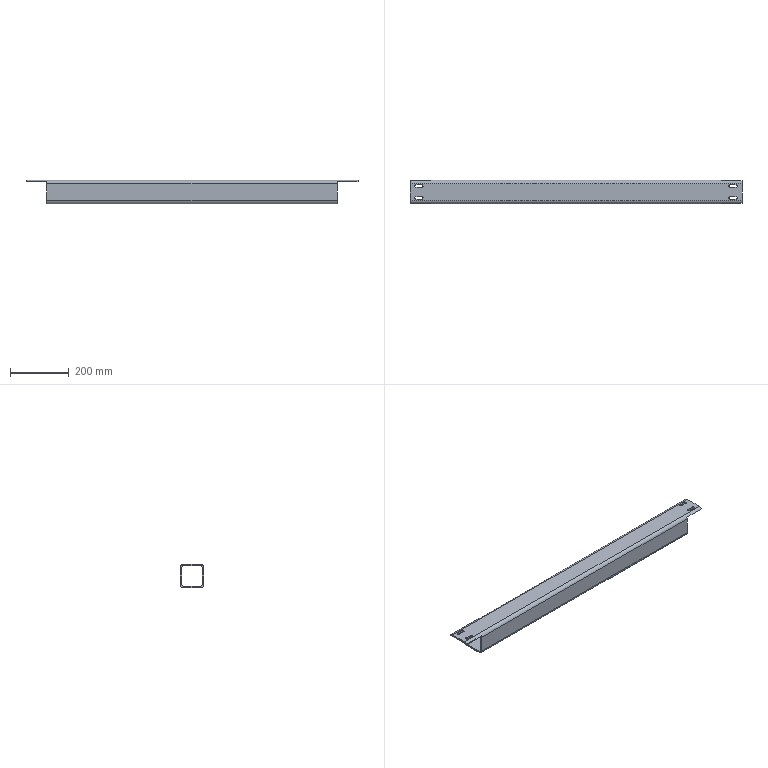Part | SolidWorks | features ICE 3, Extrusion 1 | 1 solid | 40 faces | box 1128 x 80 x 80 mm | volume 1646266 mm3 | cylinder 20 | plane 20 | commonest cylinder face diameters 8.5 x12 11.429 x4 22.857 x4
STEP:
#1=CARTESIAN_POINT('',(-439.75,-20.,34.286));
#2=VERTEX_POINT('',#1);
#3=CARTESIAN_POINT('',(-444.,-15.75,34.286));
#4=VERTEX_POINT('',#3);
#5=CARTESIAN_POINT('',(-444.,-20.,34.286));
#6=DIRECTION('',(0.,0.,1.));
#7=DIRECTION('',(1.,0.,0.));
#8=AXIS2_PLACEMENT_3D('',#5,#6,#7);
#9=CIRCLE('',#8,4.25);
#10=EDGE_CURVE('',#2,#4,#9,.T.);
#11=ORIENTED_EDGE('',*,*,#10,.F.);
#12=CARTESIAN_POINT('',(-439.75,-20.,40.));
#13=VERTEX_POINT('',#12);
#14=CARTESIAN_POINT('',(-439.75,-20.,-30.));
#15=DIRECTION('',(0.,0.,1.));
#16=VECTOR('',#15,1000.);
#17=LINE('',#14,#16);
#18=EDGE_CURVE('',#2,#13,#17,.T.);
#19=ORIENTED_EDGE('',*,*,#18,.T.);
#20=CARTESIAN_POINT('',(-444.,-15.75,40.));
#21=VERTEX_POINT('',#20);
#22=CARTESIAN_POINT('',(-444.,-20.,40.));
#23=DIRECTION('',(0.,0.,1.));
#24=DIRECTION('',(-1.,0.,0.));
#25=AXIS2_PLACEMENT_3D('',#22,#23,#24);
#26=CIRCLE('',#25,4.25);
#27=EDGE_CURVE('',#13,#21,#26,.T.);
#28=ORIENTED_EDGE('',*,*,#27,.T.);
#29=CARTESIAN_POINT('',(-444.,-15.75,-30.));
#30=DIRECTION('',(0.,0.,1.));
#31=VECTOR('',#30,1000.);
#32=LINE('',#29,#31);
#33=EDGE_CURVE('',#4,#21,#32,.T.);
#34=ORIENTED_EDGE('',*,*,#33,.F.);
#35=EDGE_LOOP('',(#11,#19,#28,#34));
#36=FACE_OUTER_BOUND('',#35,.T.);
#37=CARTESIAN_POINT('',(-444.,-20.,-30.));
#38=DIRECTION('',(0.,0.,1.));
#39=DIRECTION('',(1.,0.,0.));
#40=AXIS2_PLACEMENT_3D('',#37,#38,#39);
#41=CYLINDRICAL_SURFACE('',#40,4.25);
#42=ADVANCED_FACE('',(#36),#41,.F.);
#43=CARTESIAN_POINT('',(628.25,20.,34.286));
#44=VERTEX_POINT('',#43);
#45=CARTESIAN_POINT('',(624.,24.25,34.286));
#46=VERTEX_POINT('',#45);
#47=CARTESIAN_POINT('',(624.,20.,34.286));
#48=DIRECTION('',(0.,0.,1.));
#49=DIRECTION('',(1.,0.,0.));
#50=AXIS2_PLACEMENT_3D('',#47,#48,#49);
#51=CIRCLE('',#50,4.25);
#52=EDGE_CURVE('',#44,#46,#51,.T.);
#53=ORIENTED_EDGE('',*,*,#52,.F.);
#54=CARTESIAN_POINT('',(628.25,20.,40.));
#55=VERTEX_POINT('',#54);
#56=CARTESIAN_POINT('',(628.25,20.,-30.));
#57=DIRECTION('',(0.,0.,1.));
#58=VECTOR('',#57,1000.);
#59=LINE('',#56,#58);
#60=EDGE_CURVE('',#44,#55,#59,.T.);
#61=ORIENTED_EDGE('',*,*,#60,.T.);
#62=CARTESIAN_POINT('',(624.,24.25,40.));
#63=VERTEX_POINT('',#62);
#64=CARTESIAN_POINT('',(624.,20.,40.));
#65=DIRECTION('',(0.,0.,1.));
#66=DIRECTION('',(1.,0.,0.));
#67=AXIS2_PLACEMENT_3D('',#64,#65,#66);
#68=CIRCLE('',#67,4.25);
#69=EDGE_CURVE('',#55,#63,#68,.T.);
#70=ORIENTED_EDGE('',*,*,#69,.T.);
#71=CARTESIAN_POINT('',(624.,24.25,-30.));
#72=DIRECTION('',(0.,0.,1.));
#73=VECTOR('',#72,1000.);
#74=LINE('',#71,#73);
#75=EDGE_CURVE('',#46,#63,#74,.T.);
#76=ORIENTED_EDGE('',*,*,#75,.F.);
#77=EDGE_LOOP('',(#53,#61,#70,#76));
#78=FACE_OUTER_BOUND('',#77,.T.);
#79=CARTESIAN_POINT('',(624.,20.,-30.));
#80=DIRECTION('',(0.,0.,1.));
#81=DIRECTION('',(1.,0.,0.));
#82=AXIS2_PLACEMENT_3D('',#79,#80,#81);
#83=CYLINDRICAL_SURFACE('',#82,4.25);
#84=ADVANCED_FACE('',(#78),#83,.F.);
#85=CARTESIAN_POINT('',(628.25,-20.,34.286));
#86=VERTEX_POINT('',#85);
#87=CARTESIAN_POINT('',(624.,-15.75,34.286));
#88=VERTEX_POINT('',#87);
#89=CARTESIAN_POINT('',(624.,-20.,34.286));
#90=DIRECTION('',(0.,0.,1.));
#91=DIRECTION('',(1.,0.,0.));
#92=AXIS2_PLACEMENT_3D('',#89,#90,#91);
#93=CIRCLE('',#92,4.25);
#94=EDGE_CURVE('',#86,#88,#93,.T.);
#95=ORIENTED_EDGE('',*,*,#94,.F.);
#96=CARTESIAN_POINT('',(628.25,-20.,40.));
#97=VERTEX_POINT('',#96);
#98=CARTESIAN_POINT('',(628.25,-20.,-30.));
#99=DIRECTION('',(0.,0.,1.));
#100=VECTOR('',#99,1000.);
#101=LINE('',#98,#100);
#102=EDGE_CURVE('',#86,#97,#101,.T.);
#103=ORIENTED_EDGE('',*,*,#102,.T.);
#104=CARTESIAN_POINT('',(624.,-15.75,40.));
#105=VERTEX_POINT('',#104);
#106=CARTESIAN_POINT('',(624.,-20.,40.));
#107=DIRECTION('',(0.,0.,1.));
#108=DIRECTION('',(-1.,0.,0.));
#109=AXIS2_PLACEMENT_3D('',#106,#107,#108);
#110=CIRCLE('',#109,4.25);
#111=EDGE_CURVE('',#97,#105,#110,.T.);
#112=ORIENTED_EDGE('',*,*,#111,.T.);
#113=CARTESIAN_POINT('',(624.,-15.75,-30.));
#114=DIRECTION('',(0.,0.,1.));
#115=VECTOR('',#114,1000.);
#116=LINE('',#113,#115);
#117=EDGE_CURVE('',#88,#105,#116,.T.);
#118=ORIENTED_EDGE('',*,*,#117,.F.);
#119=EDGE_LOOP('',(#95,#103,#112,#118));
#120=FACE_OUTER_BOUND('',#119,.T.);
#121=CARTESIAN_POINT('',(624.,-20.,-30.));
#122=DIRECTION('',(0.,0.,1.));
#123=DIRECTION('',(1.,0.,0.));
#124=AXIS2_PLACEMENT_3D('',#121,#122,#123);
#125=CYLINDRICAL_SURFACE('',#124,4.25);
#126=ADVANCED_FACE('',(#120),#125,.F.);
#127=CARTESIAN_POINT('',(-439.75,20.,34.286));
#128=VERTEX_POINT('',#127);
#129=CARTESIAN_POINT('',(-444.,24.25,34.286));
#130=VERTEX_POINT('',#129);
#131=CARTESIAN_POINT('',(-444.,20.,34.286));
#132=DIRECTION('',(0.,0.,1.));
#133=DIRECTION('',(1.,0.,0.));
#134=AXIS2_PLACEMENT_3D('',#131,#132,#133);
#135=CIRCLE('',#134,4.25);
#136=EDGE_CURVE('',#128,#130,#135,.T.);
#137=ORIENTED_EDGE('',*,*,#136,.F.);
#138=CARTESIAN_POINT('',(-439.75,20.,40.));
#139=VERTEX_POINT('',#138);
#140=CARTESIAN_POINT('',(-439.75,20.,-30.));
#141=DIRECTION('',(0.,0.,1.));
#142=VECTOR('',#141,1000.);
#143=LINE('',#140,#142);
#144=EDGE_CURVE('',#128,#139,#143,.T.);
#145=ORIENTED_EDGE('',*,*,#144,.T.);
#146=CARTESIAN_POINT('',(-444.,24.25,40.));
#147=VERTEX_POINT('',#146);
#148=CARTESIAN_POINT('',(-444.,20.,40.));
#149=DIRECTION('',(0.,0.,1.));
#150=DIRECTION('',(1.,0.,0.));
#151=AXIS2_PLACEMENT_3D('',#148,#149,#150);
#152=CIRCLE('',#151,4.25);
#153=EDGE_CURVE('',#139,#147,#152,.T.);
#154=ORIENTED_EDGE('',*,*,#153,.T.);
#155=CARTESIAN_POINT('',(-444.,24.25,-30.));
#156=DIRECTION('',(0.,0.,1.));
#157=VECTOR('',#156,1000.);
#158=LINE('',#155,#157);
#159=EDGE_CURVE('',#130,#147,#158,.T.);
#160=ORIENTED_EDGE('',*,*,#159,.F.);
#161=EDGE_LOOP('',(#137,#145,#154,#160));
#162=FACE_OUTER_BOUND('',#161,.T.);
#163=CARTESIAN_POINT('',(-444.,20.,-30.));
#164=DIRECTION('',(0.,0.,1.));
#165=DIRECTION('',(1.,0.,0.));
#166=AXIS2_PLACEMENT_3D('',#163,#164,#165);
#167=CYLINDRICAL_SURFACE('',#166,4.25);
#168=ADVANCED_FACE('',(#162),#167,.F.);
#169=CARTESIAN_POINT('',(-414.,38.469,34.286));
#170=VERTEX_POINT('',#169);
#171=CARTESIAN_POINT('',(-414.,28.571,34.286));
#172=VERTEX_POINT('',#171);
#173=CARTESIAN_POINT('',(-414.,-28.571,34.286));
#174=DIRECTION('',(0.,-1.,0.));
#175=VECTOR('',#174,1000.);
#176=LINE('',#173,#175);
#177=EDGE_CURVE('',#170,#172,#176,.T.);
#178=ORIENTED_EDGE('',*,*,#177,.F.);
#179=CARTESIAN_POINT('',(-414.,40.,28.571));
#180=VERTEX_POINT('',#179);
#181=CARTESIAN_POINT('',(-414.,28.571,28.571));
#182=DIRECTION('',(1.,0.,0.));
#183=DIRECTION('',(0.,0.,-1.));
#184=AXIS2_PLACEMENT_3D('',#181,#182,#183);
#185=CIRCLE('',#184,11.429);
#186=EDGE_CURVE('',#180,#170,#185,.T.);
#187=ORIENTED_EDGE('',*,*,#186,.F.);
#188=CARTESIAN_POINT('',(-414.,40.,-28.571));
#189=VERTEX_POINT('',#188);
#190=CARTESIAN_POINT('',(-414.,40.,-28.571));
#191=DIRECTION('',(0.,0.,1.));
#192=VECTOR('',#191,1000.);
#193=LINE('',#190,#192);
#194=EDGE_CURVE('',#189,#180,#193,.T.);
#195=ORIENTED_EDGE('',*,*,#194,.F.);
#196=CARTESIAN_POINT('',(-414.,28.571,-40.));
#197=VERTEX_POINT('',#196);
#198=CARTESIAN_POINT('',(-414.,28.571,-28.571));
#199=DIRECTION('',(1.,0.,0.));
#200=DIRECTION('',(0.,0.,-1.));
#201=AXIS2_PLACEMENT_3D('',#198,#199,#200);
#202=CIRCLE('',#201,11.429);
#203=EDGE_CURVE('',#197,#189,#202,.T.);
#204=ORIENTED_EDGE('',*,*,#203,.F.);
#205=CARTESIAN_POINT('',(-414.,-28.571,-40.));
#206=VERTEX_POINT('',#205);
#207=CARTESIAN_POINT('',(-414.,-28.571,-40.));
#208=DIRECTION('',(0.,1.,0.));
#209=VECTOR('',#208,1000.);
#210=LINE('',#207,#209);
#211=EDGE_CURVE('',#206,#197,#210,.T.);
#212=ORIENTED_EDGE('',*,*,#211,.F.);
#213=CARTESIAN_POINT('',(-414.,-40.,-28.571));
#214=VERTEX_POINT('',#213);
#215=CARTESIAN_POINT('',(-414.,-28.571,-28.571));
#216=DIRECTION('',(1.,0.,0.));
#217=DIRECTION('',(0.,0.,-1.));
#218=AXIS2_PLACEMENT_3D('',#215,#216,#217);
#219=CIRCLE('',#218,11.429);
#220=EDGE_CURVE('',#214,#206,#219,.T.);
#221=ORIENTED_EDGE('',*,*,#220,.F.);
#222=CARTESIAN_POINT('',(-414.,-40.,28.571));
#223=VERTEX_POINT('',#222);
#224=CARTESIAN_POINT('',(-414.,-40.,28.571));
#225=DIRECTION('',(0.,0.,-1.));
#226=VECTOR('',#225,1000.);
#227=LINE('',#224,#226);
#228=EDGE_CURVE('',#223,#214,#227,.T.);
#229=ORIENTED_EDGE('',*,*,#228,.F.);
#230=CARTESIAN_POINT('',(-414.,-38.469,34.286));
#231=VERTEX_POINT('',#230);
#232=CARTESIAN_POINT('',(-414.,-28.571,28.571));
#233=DIRECTION('',(1.,0.,0.));
#234=DIRECTION('',(0.,0.,-1.));
#235=AXIS2_PLACEMENT_3D('',#232,#233,#234);
#236=CIRCLE('',#235,11.429);
#237=EDGE_CURVE('',#231,#223,#236,.T.);
#238=ORIENTED_EDGE('',*,*,#237,.F.);
#239=CARTESIAN_POINT('',(-414.,-28.571,34.286));
#240=VERTEX_POINT('',#239);
#241=CARTESIAN_POINT('',(-414.,-28.571,34.286));
#242=DIRECTION('',(0.,-1.,0.));
#243=VECTOR('',#242,1000.);
#244=LINE('',#241,#243);
#245=EDGE_CURVE('',#240,#231,#244,.T.);
#246=ORIENTED_EDGE('',*,*,#245,.F.);
#247=CARTESIAN_POINT('',(-414.,-34.286,28.571));
#248=VERTEX_POINT('',#247);
#249=CARTESIAN_POINT('',(-414.,-28.571,28.571));
#250=DIRECTION('',(1.,0.,0.));
#251=DIRECTION('',(0.,0.,1.));
#252=AXIS2_PLACEMENT_3D('',#249,#250,#251);
#253=CIRCLE('',#252,5.714);
#254=EDGE_CURVE('',#240,#248,#253,.T.);
#255=ORIENTED_EDGE('',*,*,#254,.T.);
#256=CARTESIAN_POINT('',(-414.,-34.286,-28.571));
#257=VERTEX_POINT('',#256);
#258=CARTESIAN_POINT('',(-414.,-34.286,-28.571));
#259=DIRECTION('',(0.,0.,-1.));
#260=VECTOR('',#259,1000.);
#261=LINE('',#258,#260);
#262=EDGE_CURVE('',#248,#257,#261,.T.);
#263=ORIENTED_EDGE('',*,*,#262,.T.);
#264=CARTESIAN_POINT('',(-414.,-28.571,-34.286));
#265=VERTEX_POINT('',#264);
#266=CARTESIAN_POINT('',(-414.,-28.571,-28.571));
#267=DIRECTION('',(1.,0.,0.));
#268=DIRECTION('',(0.,0.,1.));
#269=AXIS2_PLACEMENT_3D('',#266,#267,#268);
#270=CIRCLE('',#269,5.714);
#271=EDGE_CURVE('',#257,#265,#270,.T.);
#272=ORIENTED_EDGE('',*,*,#271,.T.);
#273=CARTESIAN_POINT('',(-414.,28.571,-34.286));
#274=VERTEX_POINT('',#273);
#275=CARTESIAN_POINT('',(-414.,28.571,-34.286));
#276=DIRECTION('',(0.,1.,0.));
#277=VECTOR('',#276,1000.);
#278=LINE('',#275,#277);
#279=EDGE_CURVE('',#265,#274,#278,.T.);
#280=ORIENTED_EDGE('',*,*,#279,.T.);
#281=CARTESIAN_POINT('',(-414.,34.286,-28.571));
#282=VERTEX_POINT('',#281);
#283=CARTESIAN_POINT('',(-414.,28.571,-28.571));
#284=DIRECTION('',(1.,0.,0.));
#285=DIRECTION('',(0.,0.,1.));
#286=AXIS2_PLACEMENT_3D('',#283,#284,#285);
#287=CIRCLE('',#286,5.714);
#288=EDGE_CURVE('',#274,#282,#287,.T.);
#289=ORIENTED_EDGE('',*,*,#288,.T.);
#290=CARTESIAN_POINT('',(-414.,34.286,28.571));
#291=VERTEX_POINT('',#290);
#292=CARTESIAN_POINT('',(-414.,34.286,28.571));
#293=DIRECTION('',(0.,0.,1.));
#294=VECTOR('',#293,1000.);
#295=LINE('',#292,#294);
#296=EDGE_CURVE('',#282,#291,#295,.T.);
#297=ORIENTED_EDGE('',*,*,#296,.T.);
#298=CARTESIAN_POINT('',(-414.,28.571,28.571));
#299=DIRECTION('',(1.,0.,0.));
#300=DIRECTION('',(0.,0.,1.));
#301=AXIS2_PLACEMENT_3D('',#298,#299,#300);
#302=CIRCLE('',#301,5.714);
#303=EDGE_CURVE('',#291,#172,#302,.T.);
#304=ORIENTED_EDGE('',*,*,#303,.T.);
#305=EDGE_LOOP('',(#178,#187,#195,#204,#212,#221,#229,#238,#246,#255,#263,#272,#280,#289,#297,#304));
#306=FACE_OUTER_BOUND('',#305,.T.);
#307=CARTESIAN_POINT('',(-414.,-28.571,-28.571));
#308=DIRECTION('',(1.,0.,0.));
#309=DIRECTION('',(0.,0.,-1.));
#310=AXIS2_PLACEMENT_3D('',#307,#308,#309);
#311=PLANE('',#310);
#312=ADVANCED_FACE('',(#306),#311,.F.);
#313=CARTESIAN_POINT('',(574.,-40.,-28.571));
#314=VERTEX_POINT('',#313);
#315=CARTESIAN_POINT('',(574.,-28.571,-40.));
#316=VERTEX_POINT('',#315);
#317=CARTESIAN_POINT('',(574.,-28.571,-28.571));
#318=DIRECTION('',(1.,0.,0.));
#319=DIRECTION('',(0.,0.,-1.));
#320=AXIS2_PLACEMENT_3D('',#317,#318,#319);
#321=CIRCLE('',#320,11.429);
#322=EDGE_CURVE('',#314,#316,#321,.T.);
#323=ORIENTED_EDGE('',*,*,#322,.F.);
#324=CARTESIAN_POINT('',(-414.,-40.,-28.571));
#325=DIRECTION('',(1.,0.,0.));
#326=VECTOR('',#325,1000.);
#327=LINE('',#324,#326);
#328=EDGE_CURVE('',#214,#314,#327,.T.);
#329=ORIENTED_EDGE('',*,*,#328,.F.);
#330=ORIENTED_EDGE('',*,*,#220,.T.);
#331=CARTESIAN_POINT('',(-414.,-28.571,-40.));
#332=DIRECTION('',(1.,0.,0.));
#333=VECTOR('',#332,1000.);
#334=LINE('',#331,#333);
#335=EDGE_CURVE('',#206,#316,#334,.T.);
#336=ORIENTED_EDGE('',*,*,#335,.T.);
#337=EDGE_LOOP('',(#323,#329,#330,#336));
#338=FACE_OUTER_BOUND('',#337,.T.);
#339=CARTESIAN_POINT('',(-414.,-28.571,-28.571));
#340=DIRECTION('',(1.,0.,0.));
#341=DIRECTION('',(0.,0.,-1.));
#342=AXIS2_PLACEMENT_3D('',#339,#340,#341);
#343=CYLINDRICAL_SURFACE('',#342,11.429);
#344=ADVANCED_FACE('',(#338),#343,.T.);
#345=CARTESIAN_POINT('',(574.,-40.,28.571));
#346=VERTEX_POINT('',#345);
#347=CARTESIAN_POINT('',(574.,-40.,28.571));
#348=DIRECTION('',(0.,0.,-1.));
#349=VECTOR('',#348,1000.);
#350=LINE('',#347,#349);
#351=EDGE_CURVE('',#346,#314,#350,.T.);
#352=ORIENTED_EDGE('',*,*,#351,.F.);
#353=CARTESIAN_POINT('',(-414.,-40.,28.571));
#354=DIRECTION('',(1.,0.,0.));
#355=VECTOR('',#354,1000.);
#356=LINE('',#353,#355);
#357=EDGE_CURVE('',#223,#346,#356,.T.);
#358=ORIENTED_EDGE('',*,*,#357,.F.);
#359=ORIENTED_EDGE('',*,*,#228,.T.);
#360=ORIENTED_EDGE('',*,*,#328,.T.);
#361=EDGE_LOOP('',(#352,#358,#359,#360));
#362=FACE_OUTER_BOUND('',#361,.T.);
#363=CARTESIAN_POINT('',(-414.,-40.,28.571));
#364=DIRECTION('',(0.,-1.,0.));
#365=DIRECTION('',(0.,0.,-1.));
#366=AXIS2_PLACEMENT_3D('',#363,#364,#365);
#367=PLANE('',#366);
#368=ADVANCED_FACE('',(#362),#367,.T.);
#369=CARTESIAN_POINT('',(574.,-38.469,34.286));
#370=VERTEX_POINT('',#369);
#371=CARTESIAN_POINT('',(574.,-28.571,28.571));
#372=DIRECTION('',(1.,0.,0.));
#373=DIRECTION('',(0.,0.,-1.));
#374=AXIS2_PLACEMENT_3D('',#371,#372,#373);
#375=CIRCLE('',#374,11.429);
#376=EDGE_CURVE('',#370,#346,#375,.T.);
#377=ORIENTED_EDGE('',*,*,#376,.F.);
#378=CARTESIAN_POINT('',(644.,-38.469,34.286));
#379=VERTEX_POINT('',#378);
#380=CARTESIAN_POINT('',(644.,-38.469,34.286));
#381=DIRECTION('',(-1.,0.,0.));
#382=VECTOR('',#381,1000.);
#383=LINE('',#380,#382);
#384=EDGE_CURVE('',#379,#370,#383,.T.);
#385=ORIENTED_EDGE('',*,*,#384,.F.);
#386=CARTESIAN_POINT('',(644.,-28.571,40.));
#387=VERTEX_POINT('',#386);
#388=CARTESIAN_POINT('',(644.,-28.571,28.571));
#389=DIRECTION('',(1.,0.,0.));
#390=DIRECTION('',(0.,0.,-1.));
#391=AXIS2_PLACEMENT_3D('',#388,#389,#390);
#392=CIRCLE('',#391,11.429);
#393=EDGE_CURVE('',#387,#379,#392,.T.);
#394=ORIENTED_EDGE('',*,*,#393,.F.);
#395=CARTESIAN_POINT('',(-484.,-28.571,40.));
#396=VERTEX_POINT('',#395);
#397=CARTESIAN_POINT('',(-414.,-28.571,40.));
#398=DIRECTION('',(1.,0.,0.));
#399=VECTOR('',#398,1000.);
#400=LINE('',#397,#399);
#401=EDGE_CURVE('',#396,#387,#400,.T.);
#402=ORIENTED_EDGE('',*,*,#401,.F.);
#403=CARTESIAN_POINT('',(-484.,-38.469,34.286));
#404=VERTEX_POINT('',#403);
#405=CARTESIAN_POINT('',(-484.,-28.571,28.571));
#406=DIRECTION('',(-1.,0.,0.));
#407=DIRECTION('',(0.,0.,1.));
#408=AXIS2_PLACEMENT_3D('',#405,#406,#407);
#409=CIRCLE('',#408,11.429);
#410=EDGE_CURVE('',#404,#396,#409,.T.);
#411=ORIENTED_EDGE('',*,*,#410,.F.);
#412=CARTESIAN_POINT('',(-484.,-38.469,34.286));
#413=DIRECTION('',(1.,0.,0.));
#414=VECTOR('',#413,1000.);
#415=LINE('',#412,#414);
#416=EDGE_CURVE('',#404,#231,#415,.T.);
#417=ORIENTED_EDGE('',*,*,#416,.T.);
#418=ORIENTED_EDGE('',*,*,#237,.T.);
#419=ORIENTED_EDGE('',*,*,#357,.T.);
#420=EDGE_LOOP('',(#377,#385,#394,#402,#411,#417,#418,#419));
#421=FACE_OUTER_BOUND('',#420,.T.);
#422=CARTESIAN_POINT('',(-414.,-28.571,28.571));
#423=DIRECTION('',(1.,0.,0.));
#424=DIRECTION('',(0.,0.,-1.));
#425=AXIS2_PLACEMENT_3D('',#422,#423,#424);
#426=CYLINDRICAL_SURFACE('',#425,11.429);
#427=ADVANCED_FACE('',(#421),#426,.T.);
#428=CARTESIAN_POINT('',(-464.,-15.75,40.));
#429=VERTEX_POINT('',#428);
#430=CARTESIAN_POINT('',(-464.,-24.25,40.));
#431=VERTEX_POINT('',#430);
#432=CARTESIAN_POINT('',(-464.,-20.,40.));
#433=DIRECTION('',(0.,0.,1.));
#434=DIRECTION('',(-1.,0.,0.));
#435=AXIS2_PLACEMENT_3D('',#432,#433,#434);
#436=CIRCLE('',#435,4.25);
#437=EDGE_CURVE('',#429,#431,#436,.T.);
#438=ORIENTED_EDGE('',*,*,#437,.F.);
#439=CARTESIAN_POINT('',(-464.,-15.75,40.));
#440=DIRECTION('',(-1.,0.,0.));
#441=VECTOR('',#440,1000.);
#442=LINE('',#439,#441);
#443=EDGE_CURVE('',#21,#429,#442,.T.);
#444=ORIENTED_EDGE('',*,*,#443,.F.);
#445=ORIENTED_EDGE('',*,*,#27,.F.);
#446=CARTESIAN_POINT('',(-444.,-24.25,40.));
#447=VERTEX_POINT('',#446);
#448=CARTESIAN_POINT('',(-444.,-20.,40.));
#449=DIRECTION('',(0.,0.,1.));
#450=DIRECTION('',(-1.,0.,0.));
#451=AXIS2_PLACEMENT_3D('',#448,#449,#450);
#452=CIRCLE('',#451,4.25);
#453=EDGE_CURVE('',#447,#13,#452,.T.);
#454=ORIENTED_EDGE('',*,*,#453,.F.);
#455=CARTESIAN_POINT('',(-464.,-24.25,40.));
#456=DIRECTION('',(1.,0.,0.));
#457=VECTOR('',#456,1000.);
#458=LINE('',#455,#457);
#459=EDGE_CURVE('',#431,#447,#458,.T.);
#460=ORIENTED_EDGE('',*,*,#459,.F.);
#461=EDGE_LOOP('',(#438,#444,#445,#454,#460));
#462=FACE_BOUND('',#461,.T.);
#463=CARTESIAN_POINT('',(604.,24.25,40.));
#464=VERTEX_POINT('',#463);
#465=CARTESIAN_POINT('',(604.,15.75,40.));
#466=VERTEX_POINT('',#465);
#467=CARTESIAN_POINT('',(604.,20.,40.));
#468=DIRECTION('',(0.,0.,1.));
#469=DIRECTION('',(1.,0.,0.));
#470=AXIS2_PLACEMENT_3D('',#467,#468,#469);
#471=CIRCLE('',#470,4.25);
#472=EDGE_CURVE('',#464,#466,#471,.T.);
#473=ORIENTED_EDGE('',*,*,#472,.F.);
#474=CARTESIAN_POINT('',(604.,24.25,40.));
#475=DIRECTION('',(-1.,0.,0.));
#476=VECTOR('',#475,1000.);
#477=LINE('',#474,#476);
#478=EDGE_CURVE('',#63,#464,#477,.T.);
#479=ORIENTED_EDGE('',*,*,#478,.F.);
#480=ORIENTED_EDGE('',*,*,#69,.F.);
#481=CARTESIAN_POINT('',(624.,15.75,40.));
#482=VERTEX_POINT('',#481);
#483=CARTESIAN_POINT('',(624.,20.,40.));
#484=DIRECTION('',(0.,0.,1.));
#485=DIRECTION('',(1.,0.,0.));
#486=AXIS2_PLACEMENT_3D('',#483,#484,#485);
#487=CIRCLE('',#486,4.25);
#488=EDGE_CURVE('',#482,#55,#487,.T.);
#489=ORIENTED_EDGE('',*,*,#488,.F.);
#490=CARTESIAN_POINT('',(604.,15.75,40.));
#491=DIRECTION('',(1.,0.,0.));
#492=VECTOR('',#491,1000.);
#493=LINE('',#490,#492);
#494=EDGE_CURVE('',#466,#482,#493,.T.);
#495=ORIENTED_EDGE('',*,*,#494,.F.);
#496=EDGE_LOOP('',(#473,#479,#480,#489,#495));
#497=FACE_BOUND('',#496,.T.);
#498=CARTESIAN_POINT('',(604.,-15.75,40.));
#499=VERTEX_POINT('',#498);
#500=CARTESIAN_POINT('',(604.,-24.25,40.));
#501=VERTEX_POINT('',#500);
#502=CARTESIAN_POINT('',(604.,-20.,40.));
#503=DIRECTION('',(0.,0.,1.));
#504=DIRECTION('',(-1.,0.,0.));
#505=AXIS2_PLACEMENT_3D('',#502,#503,#504);
#506=CIRCLE('',#505,4.25);
#507=EDGE_CURVE('',#499,#501,#506,.T.);
#508=ORIENTED_EDGE('',*,*,#507,.F.);
#509=CARTESIAN_POINT('',(604.,-15.75,40.));
#510=DIRECTION('',(-1.,0.,0.));
#511=VECTOR('',#510,1000.);
#512=LINE('',#509,#511);
#513=EDGE_CURVE('',#105,#499,#512,.T.);
#514=ORIENTED_EDGE('',*,*,#513,.F.);
#515=ORIENTED_EDGE('',*,*,#111,.F.);
#516=CARTESIAN_POINT('',(624.,-24.25,40.));
#517=VERTEX_POINT('',#516);
#518=CARTESIAN_POINT('',(624.,-20.,40.));
#519=DIRECTION('',(0.,0.,1.));
#520=DIRECTION('',(-1.,0.,0.));
#521=AXIS2_PLACEMENT_3D('',#518,#519,#520);
#522=CIRCLE('',#521,4.25);
#523=EDGE_CURVE('',#517,#97,#522,.T.);
#524=ORIENTED_EDGE('',*,*,#523,.F.);
#525=CARTESIAN_POINT('',(604.,-24.25,40.));
#526=DIRECTION('',(1.,0.,0.));
#527=VECTOR('',#526,1000.);
#528=LINE('',#525,#527);
#529=EDGE_CURVE('',#501,#517,#528,.T.);
#530=ORIENTED_EDGE('',*,*,#529,.F.);
#531=EDGE_LOOP('',(#508,#514,#515,#524,#530));
#532=FACE_BOUND('',#531,.T.);
#533=CARTESIAN_POINT('',(-464.,24.25,40.));
#534=VERTEX_POINT('',#533);
#535=CARTESIAN_POINT('',(-464.,15.75,40.));
#536=VERTEX_POINT('',#535);
#537=CARTESIAN_POINT('',(-464.,20.,40.));
#538=DIRECTION('',(0.,0.,1.));
#539=DIRECTION('',(1.,0.,0.));
#540=AXIS2_PLACEMENT_3D('',#537,#538,#539);
#541=CIRCLE('',#540,4.25);
#542=EDGE_CURVE('',#534,#536,#541,.T.);
#543=ORIENTED_EDGE('',*,*,#542,.F.);
#544=CARTESIAN_POINT('',(-464.,24.25,40.));
#545=DIRECTION('',(-1.,0.,0.));
#546=VECTOR('',#545,1000.);
#547=LINE('',#544,#546);
#548=EDGE_CURVE('',#147,#534,#547,.T.);
#549=ORIENTED_EDGE('',*,*,#548,.F.);
#550=ORIENTED_EDGE('',*,*,#153,.F.);
#551=CARTESIAN_POINT('',(-444.,15.75,40.));
#552=VERTEX_POINT('',#551);
#553=CARTESIAN_POINT('',(-444.,20.,40.));
#554=DIRECTION('',(0.,0.,1.));
#555=DIRECTION('',(1.,0.,0.));
#556=AXIS2_PLACEMENT_3D('',#553,#554,#555);
#557=CIRCLE('',#556,4.25);
#558=EDGE_CURVE('',#552,#139,#557,.T.);
#559=ORIENTED_EDGE('',*,*,#558,.F.);
#560=CARTESIAN_POINT('',(-464.,15.75,40.));
#561=DIRECTION('',(1.,0.,0.));
#562=VECTOR('',#561,1000.);
#563=LINE('',#560,#562);
#564=EDGE_CURVE('',#536,#552,#563,.T.);
#565=ORIENTED_EDGE('',*,*,#564,.F.);
#566=EDGE_LOOP('',(#543,#549,#550,#559,#565));
#567=FACE_BOUND('',#566,.T.);
#568=ORIENTED_EDGE('',*,*,#401,.T.);
#569=CARTESIAN_POINT('',(644.,28.571,40.));
#570=VERTEX_POINT('',#569);
#571=CARTESIAN_POINT('',(644.,28.571,40.));
#572=DIRECTION('',(0.,-1.,0.));
#573=VECTOR('',#572,1000.);
#574=LINE('',#571,#573);
#575=EDGE_CURVE('',#570,#387,#574,.T.);
#576=ORIENTED_EDGE('',*,*,#575,.F.);
#577=CARTESIAN_POINT('',(-484.,28.571,40.));
#578=VERTEX_POINT('',#577);
#579=CARTESIAN_POINT('',(-414.,28.571,40.));
#580=DIRECTION('',(1.,0.,0.));
#581=VECTOR('',#580,1000.);
#582=LINE('',#579,#581);
#583=EDGE_CURVE('',#578,#570,#582,.T.);
#584=ORIENTED_EDGE('',*,*,#583,.F.);
#585=CARTESIAN_POINT('',(-484.,-28.571,40.));
#586=DIRECTION('',(0.,1.,0.));
#587=VECTOR('',#586,1000.);
#588=LINE('',#585,#587);
#589=EDGE_CURVE('',#396,#578,#588,.T.);
#590=ORIENTED_EDGE('',*,*,#589,.F.);
#591=EDGE_LOOP('',(#568,#576,#584,#590));
#592=FACE_OUTER_BOUND('',#591,.T.);
#593=CARTESIAN_POINT('',(-414.,28.571,40.));
#594=DIRECTION('',(0.,0.,1.));
#595=DIRECTION('',(1.,0.,0.));
#596=AXIS2_PLACEMENT_3D('',#593,#594,#595);
#597=PLANE('',#596);
#598=ADVANCED_FACE('',(#462,#497,#532,#567,#592),#597,.T.);
#599=CARTESIAN_POINT('',(574.,40.,28.571));
#600=VERTEX_POINT('',#599);
#601=CARTESIAN_POINT('',(574.,38.469,34.286));
#602=VERTEX_POINT('',#601);
#603=CARTESIAN_POINT('',(574.,28.571,28.571));
#604=DIRECTION('',(1.,0.,0.));
#605=DIRECTION('',(0.,0.,-1.));
#606=AXIS2_PLACEMENT_3D('',#603,#604,#605);
#607=CIRCLE('',#606,11.429);
#608=EDGE_CURVE('',#600,#602,#607,.T.);
#609=ORIENTED_EDGE('',*,*,#608,.F.);
#610=CARTESIAN_POINT('',(-414.,40.,28.571));
#611=DIRECTION('',(1.,0.,0.));
#612=VECTOR('',#611,1000.);
#613=LINE('',#610,#612);
#614=EDGE_CURVE('',#180,#600,#613,.T.);
#615=ORIENTED_EDGE('',*,*,#614,.F.);
#616=ORIENTED_EDGE('',*,*,#186,.T.);
#617=CARTESIAN_POINT('',(-484.,38.469,34.286));
#618=VERTEX_POINT('',#617);
#619=CARTESIAN_POINT('',(-484.,38.469,34.286));
#620=DIRECTION('',(1.,0.,0.));
#621=VECTOR('',#620,1000.);
#622=LINE('',#619,#621);
#623=EDGE_CURVE('',#618,#170,#622,.T.);
#624=ORIENTED_EDGE('',*,*,#623,.F.);
#625=CARTESIAN_POINT('',(-484.,28.571,28.571));
#626=DIRECTION('',(-1.,0.,0.));
#627=DIRECTION('',(0.,0.,1.));
#628=AXIS2_PLACEMENT_3D('',#625,#626,#627);
#629=CIRCLE('',#628,11.429);
#630=EDGE_CURVE('',#578,#618,#629,.T.);
#631=ORIENTED_EDGE('',*,*,#630,.F.);
#632=ORIENTED_EDGE('',*,*,#583,.T.);
#633=CARTESIAN_POINT('',(644.,38.469,34.286));
#634=VERTEX_POINT('',#633);
#635=CARTESIAN_POINT('',(644.,28.571,28.571));
#636=DIRECTION('',(1.,0.,0.));
#637=DIRECTION('',(0.,0.,-1.));
#638=AXIS2_PLACEMENT_3D('',#635,#636,#637);
#639=CIRCLE('',#638,11.429);
#640=EDGE_CURVE('',#634,#570,#639,.T.);
#641=ORIENTED_EDGE('',*,*,#640,.F.);
#642=CARTESIAN_POINT('',(644.,38.469,34.286));
#643=DIRECTION('',(-1.,0.,0.));
#644=VECTOR('',#643,1000.);
#645=LINE('',#642,#644);
#646=EDGE_CURVE('',#634,#602,#645,.T.);
#647=ORIENTED_EDGE('',*,*,#646,.T.);
#648=EDGE_LOOP('',(#609,#615,#616,#624,#631,#632,#641,#647));
#649=FACE_OUTER_BOUND('',#648,.T.);
#650=CARTESIAN_POINT('',(-414.,28.571,28.571));
#651=DIRECTION('',(1.,0.,0.));
#652=DIRECTION('',(0.,0.,-1.));
#653=AXIS2_PLACEMENT_3D('',#650,#651,#652);
#654=CYLINDRICAL_SURFACE('',#653,11.429);
#655=ADVANCED_FACE('',(#649),#654,.T.);
#656=CARTESIAN_POINT('',(574.,40.,-28.571));
#657=VERTEX_POINT('',#656);
#658=CARTESIAN_POINT('',(574.,40.,-28.571));
#659=DIRECTION('',(0.,0.,1.));
#660=VECTOR('',#659,1000.);
#661=LINE('',#658,#660);
#662=EDGE_CURVE('',#657,#600,#661,.T.);
#663=ORIENTED_EDGE('',*,*,#662,.F.);
#664=CARTESIAN_POINT('',(-414.,40.,-28.571));
#665=DIRECTION('',(1.,0.,0.));
#666=VECTOR('',#665,1000.);
#667=LINE('',#664,#666);
#668=EDGE_CURVE('',#189,#657,#667,.T.);
#669=ORIENTED_EDGE('',*,*,#668,.F.);
#670=ORIENTED_EDGE('',*,*,#194,.T.);
#671=ORIENTED_EDGE('',*,*,#614,.T.);
#672=EDGE_LOOP('',(#663,#669,#670,#671));
#673=FACE_OUTER_BOUND('',#672,.T.);
#674=CARTESIAN_POINT('',(-414.,40.,-28.571));
#675=DIRECTION('',(0.,1.,0.));
#676=DIRECTION('',(0.,0.,1.));
#677=AXIS2_PLACEMENT_3D('',#674,#675,#676);
#678=PLANE('',#677);
#679=ADVANCED_FACE('',(#673),#678,.T.);
#680=CARTESIAN_POINT('',(574.,28.571,-40.));
#681=VERTEX_POINT('',#680);
#682=CARTESIAN_POINT('',(574.,28.571,-28.571));
#683=DIRECTION('',(1.,0.,0.));
#684=DIRECTION('',(0.,0.,-1.));
#685=AXIS2_PLACEMENT_3D('',#682,#683,#684);
#686=CIRCLE('',#685,11.429);
#687=EDGE_CURVE('',#681,#657,#686,.T.);
#688=ORIENTED_EDGE('',*,*,#687,.F.);
#689=CARTESIAN_POINT('',(-414.,28.571,-40.));
#690=DIRECTION('',(1.,0.,0.));
#691=VECTOR('',#690,1000.);
#692=LINE('',#689,#691);
#693=EDGE_CURVE('',#197,#681,#692,.T.);
#694=ORIENTED_EDGE('',*,*,#693,.F.);
#695=ORIENTED_EDGE('',*,*,#203,.T.);
#696=ORIENTED_EDGE('',*,*,#668,.T.);
#697=EDGE_LOOP('',(#688,#694,#695,#696));
#698=FACE_OUTER_BOUND('',#697,.T.);
#699=CARTESIAN_POINT('',(-414.,28.571,-28.571));
#700=DIRECTION('',(1.,0.,0.));
#701=DIRECTION('',(0.,0.,-1.));
#702=AXIS2_PLACEMENT_3D('',#699,#700,#701);
#703=CYLINDRICAL_SURFACE('',#702,11.429);
#704=ADVANCED_FACE('',(#698),#703,.T.);
#705=CARTESIAN_POINT('',(574.,-28.571,-40.));
#706=DIRECTION('',(0.,1.,0.));
#707=VECTOR('',#706,1000.);
#708=LINE('',#705,#707);
#709=EDGE_CURVE('',#316,#681,#708,.T.);
#710=ORIENTED_EDGE('',*,*,#709,.F.);
#711=ORIENTED_EDGE('',*,*,#335,.F.);
#712=ORIENTED_EDGE('',*,*,#211,.T.);
#713=ORIENTED_EDGE('',*,*,#693,.T.);
#714=EDGE_LOOP('',(#710,#711,#712,#713));
#715=FACE_OUTER_BOUND('',#714,.T.);
#716=CARTESIAN_POINT('',(-414.,-28.571,-40.));
#717=DIRECTION('',(0.,0.,-1.));
#718=DIRECTION('',(-1.,0.,0.));
#719=AXIS2_PLACEMENT_3D('',#716,#717,#718);
#720=PLANE('',#719);
#721=ADVANCED_FACE('',(#715),#720,.T.);
#722=CARTESIAN_POINT('',(574.,-28.571,34.286));
#723=VERTEX_POINT('',#722);
#724=CARTESIAN_POINT('',(574.,28.571,34.286));
#725=DIRECTION('',(0.,1.,0.));
#726=VECTOR('',#725,1000.);
#727=LINE('',#724,#726);
#728=EDGE_CURVE('',#370,#723,#727,.T.);
#729=ORIENTED_EDGE('',*,*,#728,.F.);
#730=ORIENTED_EDGE('',*,*,#376,.T.);
#731=ORIENTED_EDGE('',*,*,#351,.T.);
#732=ORIENTED_EDGE('',*,*,#322,.T.);
#733=ORIENTED_EDGE('',*,*,#709,.T.);
#734=ORIENTED_EDGE('',*,*,#687,.T.);
#735=ORIENTED_EDGE('',*,*,#662,.T.);
#736=ORIENTED_EDGE('',*,*,#608,.T.);
#737=CARTESIAN_POINT('',(574.,28.571,34.286));
#738=VERTEX_POINT('',#737);
#739=CARTESIAN_POINT('',(574.,28.571,34.286));
#740=DIRECTION('',(0.,1.,0.));
#741=VECTOR('',#740,1000.);
#742=LINE('',#739,#741);
#743=EDGE_CURVE('',#738,#602,#742,.T.);
#744=ORIENTED_EDGE('',*,*,#743,.F.);
#745=CARTESIAN_POINT('',(574.,34.286,28.571));
#746=VERTEX_POINT('',#745);
#747=CARTESIAN_POINT('',(574.,28.571,28.571));
#748=DIRECTION('',(1.,0.,0.));
#749=DIRECTION('',(0.,0.,1.));
#750=AXIS2_PLACEMENT_3D('',#747,#748,#749);
#751=CIRCLE('',#750,5.714);
#752=EDGE_CURVE('',#746,#738,#751,.T.);
#753=ORIENTED_EDGE('',*,*,#752,.F.);
#754=CARTESIAN_POINT('',(574.,34.286,-28.571));
#755=VERTEX_POINT('',#754);
#756=CARTESIAN_POINT('',(574.,34.286,28.571));
#757=DIRECTION('',(0.,0.,1.));
#758=VECTOR('',#757,1000.);
#759=LINE('',#756,#758);
#760=EDGE_CURVE('',#755,#746,#759,.T.);
#761=ORIENTED_EDGE('',*,*,#760,.F.);
#762=CARTESIAN_POINT('',(574.,28.571,-34.286));
#763=VERTEX_POINT('',#762);
#764=CARTESIAN_POINT('',(574.,28.571,-28.571));
#765=DIRECTION('',(1.,0.,0.));
#766=DIRECTION('',(0.,0.,1.));
#767=AXIS2_PLACEMENT_3D('',#764,#765,#766);
#768=CIRCLE('',#767,5.714);
#769=EDGE_CURVE('',#763,#755,#768,.T.);
#770=ORIENTED_EDGE('',*,*,#769,.F.);
#771=CARTESIAN_POINT('',(574.,-28.571,-34.286));
#772=VERTEX_POINT('',#771);
#773=CARTESIAN_POINT('',(574.,28.571,-34.286));
#774=DIRECTION('',(0.,1.,0.));
#775=VECTOR('',#774,1000.);
#776=LINE('',#773,#775);
#777=EDGE_CURVE('',#772,#763,#776,.T.);
#778=ORIENTED_EDGE('',*,*,#777,.F.);
#779=CARTESIAN_POINT('',(574.,-34.286,-28.571));
#780=VERTEX_POINT('',#779);
#781=CARTESIAN_POINT('',(574.,-28.571,-28.571));
#782=DIRECTION('',(1.,0.,0.));
#783=DIRECTION('',(0.,0.,1.));
#784=AXIS2_PLACEMENT_3D('',#781,#782,#783);
#785=CIRCLE('',#784,5.714);
#786=EDGE_CURVE('',#780,#772,#785,.T.);
#787=ORIENTED_EDGE('',*,*,#786,.F.);
#788=CARTESIAN_POINT('',(574.,-34.286,28.571));
#789=VERTEX_POINT('',#788);
#790=CARTESIAN_POINT('',(574.,-34.286,-28.571));
#791=DIRECTION('',(0.,0.,-1.));
#792=VECTOR('',#791,1000.);
#793=LINE('',#790,#792);
#794=EDGE_CURVE('',#789,#780,#793,.T.);
#795=ORIENTED_EDGE('',*,*,#794,.F.);
#796=CARTESIAN_POINT('',(574.,-28.571,28.571));
#797=DIRECTION('',(1.,0.,0.));
#798=DIRECTION('',(0.,0.,1.));
#799=AXIS2_PLACEMENT_3D('',#796,#797,#798);
#800=CIRCLE('',#799,5.714);
#801=EDGE_CURVE('',#723,#789,#800,.T.);
#802=ORIENTED_EDGE('',*,*,#801,.F.);
#803=EDGE_LOOP('',(#729,#730,#731,#732,#733,#734,#735,#736,#744,#753,#761,#770,#778,#787,#795,#802));
#804=FACE_OUTER_BOUND('',#803,.T.);
#805=CARTESIAN_POINT('',(574.,-28.571,-28.571));
#806=DIRECTION('',(1.,0.,0.));
#807=DIRECTION('',(0.,0.,-1.));
#808=AXIS2_PLACEMENT_3D('',#805,#806,#807);
#809=PLANE('',#808);
#810=ADVANCED_FACE('',(#804),#809,.T.);
#811=ORIENTED_EDGE('',*,*,#801,.T.);
#812=CARTESIAN_POINT('',(-414.,-34.286,28.571));
#813=DIRECTION('',(1.,0.,0.));
#814=VECTOR('',#813,1000.);
#815=LINE('',#812,#814);
#816=EDGE_CURVE('',#248,#789,#815,.T.);
#817=ORIENTED_EDGE('',*,*,#816,.F.);
#818=ORIENTED_EDGE('',*,*,#254,.F.);
#819=CARTESIAN_POINT('',(-414.,-28.571,34.286));
#820=DIRECTION('',(1.,0.,0.));
#821=VECTOR('',#820,1000.);
#822=LINE('',#819,#821);
#823=EDGE_CURVE('',#240,#723,#822,.T.);
#824=ORIENTED_EDGE('',*,*,#823,.T.);
#825=EDGE_LOOP('',(#811,#817,#818,#824));
#826=FACE_OUTER_BOUND('',#825,.T.);
#827=CARTESIAN_POINT('',(-414.,-28.571,28.571));
#828=DIRECTION('',(1.,0.,0.));
#829=DIRECTION('',(0.,0.,-1.));
#830=AXIS2_PLACEMENT_3D('',#827,#828,#829);
#831=CYLINDRICAL_SURFACE('',#830,5.714);
#832=ADVANCED_FACE('',(#826),#831,.F.);
#833=CARTESIAN_POINT('',(-464.,-15.75,34.286));
#834=VERTEX_POINT('',#833);
#835=CARTESIAN_POINT('',(-414.,-15.75,34.286));
#836=DIRECTION('',(-1.,0.,0.));
#837=VECTOR('',#836,1000.);
#838=LINE('',#835,#837);
#839=EDGE_CURVE('',#4,#834,#838,.T.);
#840=ORIENTED_EDGE('',*,*,#839,.T.);
#841=CARTESIAN_POINT('',(-464.,-24.25,34.286));
#842=VERTEX_POINT('',#841);
#843=CARTESIAN_POINT('',(-464.,-20.,34.286));
#844=DIRECTION('',(0.,0.,1.));
#845=DIRECTION('',(1.,0.,0.));
#846=AXIS2_PLACEMENT_3D('',#843,#844,#845);
#847=CIRCLE('',#846,4.25);
#848=EDGE_CURVE('',#834,#842,#847,.T.);
#849=ORIENTED_EDGE('',*,*,#848,.T.);
#850=CARTESIAN_POINT('',(-444.,-24.25,34.286));
#851=VERTEX_POINT('',#850);
#852=CARTESIAN_POINT('',(-414.,-24.25,34.286));
#853=DIRECTION('',(1.,0.,0.));
#854=VECTOR('',#853,1000.);
#855=LINE('',#852,#854);
#856=EDGE_CURVE('',#842,#851,#855,.T.);
#857=ORIENTED_EDGE('',*,*,#856,.T.);
#858=CARTESIAN_POINT('',(-444.,-20.,34.286));
#859=DIRECTION('',(0.,0.,1.));
#860=DIRECTION('',(1.,0.,0.));
#861=AXIS2_PLACEMENT_3D('',#858,#859,#860);
#862=CIRCLE('',#861,4.25);
#863=EDGE_CURVE('',#851,#2,#862,.T.);
#864=ORIENTED_EDGE('',*,*,#863,.T.);
#865=ORIENTED_EDGE('',*,*,#10,.T.);
#866=EDGE_LOOP('',(#840,#849,#857,#864,#865));
#867=FACE_BOUND('',#866,.T.);
#868=CARTESIAN_POINT('',(604.,24.25,34.286));
#869=VERTEX_POINT('',#868);
#870=CARTESIAN_POINT('',(-414.,24.25,34.286));
#871=DIRECTION('',(-1.,0.,0.));
#872=VECTOR('',#871,1000.);
#873=LINE('',#870,#872);
#874=EDGE_CURVE('',#46,#869,#873,.T.);
#875=ORIENTED_EDGE('',*,*,#874,.T.);
#876=CARTESIAN_POINT('',(604.,15.75,34.286));
#877=VERTEX_POINT('',#876);
#878=CARTESIAN_POINT('',(604.,20.,34.286));
#879=DIRECTION('',(0.,0.,1.));
#880=DIRECTION('',(1.,0.,0.));
#881=AXIS2_PLACEMENT_3D('',#878,#879,#880);
#882=CIRCLE('',#881,4.25);
#883=EDGE_CURVE('',#869,#877,#882,.T.);
#884=ORIENTED_EDGE('',*,*,#883,.T.);
#885=CARTESIAN_POINT('',(624.,15.75,34.286));
#886=VERTEX_POINT('',#885);
#887=CARTESIAN_POINT('',(-414.,15.75,34.286));
#888=DIRECTION('',(1.,0.,0.));
#889=VECTOR('',#888,1000.);
#890=LINE('',#887,#889);
#891=EDGE_CURVE('',#877,#886,#890,.T.);
#892=ORIENTED_EDGE('',*,*,#891,.T.);
#893=CARTESIAN_POINT('',(624.,20.,34.286));
#894=DIRECTION('',(0.,0.,1.));
#895=DIRECTION('',(1.,0.,0.));
#896=AXIS2_PLACEMENT_3D('',#893,#894,#895);
#897=CIRCLE('',#896,4.25);
#898=EDGE_CURVE('',#886,#44,#897,.T.);
#899=ORIENTED_EDGE('',*,*,#898,.T.);
#900=ORIENTED_EDGE('',*,*,#52,.T.);
#901=EDGE_LOOP('',(#875,#884,#892,#899,#900));
#902=FACE_BOUND('',#901,.T.);
#903=CARTESIAN_POINT('',(604.,-15.75,34.286));
#904=VERTEX_POINT('',#903);
#905=CARTESIAN_POINT('',(-414.,-15.75,34.286));
#906=DIRECTION('',(-1.,0.,0.));
#907=VECTOR('',#906,1000.);
#908=LINE('',#905,#907);
#909=EDGE_CURVE('',#88,#904,#908,.T.);
#910=ORIENTED_EDGE('',*,*,#909,.T.);
#911=CARTESIAN_POINT('',(604.,-24.25,34.286));
#912=VERTEX_POINT('',#911);
#913=CARTESIAN_POINT('',(604.,-20.,34.286));
#914=DIRECTION('',(0.,0.,1.));
#915=DIRECTION('',(1.,0.,0.));
#916=AXIS2_PLACEMENT_3D('',#913,#914,#915);
#917=CIRCLE('',#916,4.25);
#918=EDGE_CURVE('',#904,#912,#917,.T.);
#919=ORIENTED_EDGE('',*,*,#918,.T.);
#920=CARTESIAN_POINT('',(624.,-24.25,34.286));
#921=VERTEX_POINT('',#920);
#922=CARTESIAN_POINT('',(-414.,-24.25,34.286));
#923=DIRECTION('',(1.,0.,0.));
#924=VECTOR('',#923,1000.);
#925=LINE('',#922,#924);
#926=EDGE_CURVE('',#912,#921,#925,.T.);
#927=ORIENTED_EDGE('',*,*,#926,.T.);
#928=CARTESIAN_POINT('',(624.,-20.,34.286));
#929=DIRECTION('',(0.,0.,1.));
#930=DIRECTION('',(1.,0.,0.));
#931=AXIS2_PLACEMENT_3D('',#928,#929,#930);
#932=CIRCLE('',#931,4.25);
#933=EDGE_CURVE('',#921,#86,#932,.T.);
#934=ORIENTED_EDGE('',*,*,#933,.T.);
#935=ORIENTED_EDGE('',*,*,#94,.T.);
#936=EDGE_LOOP('',(#910,#919,#927,#934,#935));
#937=FACE_BOUND('',#936,.T.);
#938=CARTESIAN_POINT('',(-464.,24.25,34.286));
#939=VERTEX_POINT('',#938);
#940=CARTESIAN_POINT('',(-414.,24.25,34.286));
#941=DIRECTION('',(-1.,0.,0.));
#942=VECTOR('',#941,1000.);
#943=LINE('',#940,#942);
#944=EDGE_CURVE('',#130,#939,#943,.T.);
#945=ORIENTED_EDGE('',*,*,#944,.T.);
#946=CARTESIAN_POINT('',(-464.,15.75,34.286));
#947=VERTEX_POINT('',#946);
#948=CARTESIAN_POINT('',(-464.,20.,34.286));
#949=DIRECTION('',(0.,0.,1.));
#950=DIRECTION('',(1.,0.,0.));
#951=AXIS2_PLACEMENT_3D('',#948,#949,#950);
#952=CIRCLE('',#951,4.25);
#953=EDGE_CURVE('',#939,#947,#952,.T.);
#954=ORIENTED_EDGE('',*,*,#953,.T.);
#955=CARTESIAN_POINT('',(-444.,15.75,34.286));
#956=VERTEX_POINT('',#955);
#957=CARTESIAN_POINT('',(-414.,15.75,34.286));
#958=DIRECTION('',(1.,0.,0.));
#959=VECTOR('',#958,1000.);
#960=LINE('',#957,#959);
#961=EDGE_CURVE('',#947,#956,#960,.T.);
#962=ORIENTED_EDGE('',*,*,#961,.T.);
#963=CARTESIAN_POINT('',(-444.,20.,34.286));
#964=DIRECTION('',(0.,0.,1.));
#965=DIRECTION('',(1.,0.,0.));
#966=AXIS2_PLACEMENT_3D('',#963,#964,#965);
#967=CIRCLE('',#966,4.25);
#968=EDGE_CURVE('',#956,#128,#967,.T.);
#969=ORIENTED_EDGE('',*,*,#968,.T.);
#970=ORIENTED_EDGE('',*,*,#136,.T.);
#971=EDGE_LOOP('',(#945,#954,#962,#969,#970));
#972=FACE_BOUND('',#971,.T.);
#973=CARTESIAN_POINT('',(-414.,28.571,34.286));
#974=DIRECTION('',(1.,0.,0.));
#975=VECTOR('',#974,1000.);
#976=LINE('',#973,#975);
#977=EDGE_CURVE('',#172,#738,#976,.T.);
#978=ORIENTED_EDGE('',*,*,#977,.T.);
#979=ORIENTED_EDGE('',*,*,#743,.T.);
#980=ORIENTED_EDGE('',*,*,#646,.F.);
#981=CARTESIAN_POINT('',(644.,-28.571,34.286));
#982=DIRECTION('',(0.,-1.,0.));
#983=VECTOR('',#982,1000.);
#984=LINE('',#981,#983);
#985=EDGE_CURVE('',#634,#379,#984,.T.);
#986=ORIENTED_EDGE('',*,*,#985,.T.);
#987=ORIENTED_EDGE('',*,*,#384,.T.);
#988=ORIENTED_EDGE('',*,*,#728,.T.);
#989=ORIENTED_EDGE('',*,*,#823,.F.);
#990=ORIENTED_EDGE('',*,*,#245,.T.);
#991=ORIENTED_EDGE('',*,*,#416,.F.);
#992=CARTESIAN_POINT('',(-484.,-28.571,34.286));
#993=DIRECTION('',(0.,-1.,0.));
#994=VECTOR('',#993,1000.);
#995=LINE('',#992,#994);
#996=EDGE_CURVE('',#618,#404,#995,.T.);
#997=ORIENTED_EDGE('',*,*,#996,.F.);
#998=ORIENTED_EDGE('',*,*,#623,.T.);
#999=ORIENTED_EDGE('',*,*,#177,.T.);
#1000=EDGE_LOOP('',(#978,#979,#980,#986,#987,#988,#989,#990,#991,#997,#998,#999));
#1001=FACE_OUTER_BOUND('',#1000,.T.);
#1002=CARTESIAN_POINT('',(-414.,-28.571,34.286));
#1003=DIRECTION('',(0.,0.,1.));
#1004=DIRECTION('',(1.,0.,0.));
#1005=AXIS2_PLACEMENT_3D('',#1002,#1003,#1004);
#1006=PLANE('',#1005);
#1007=ADVANCED_FACE('',(#867,#902,#937,#972,#1001),#1006,.F.);
#1008=ORIENTED_EDGE('',*,*,#752,.T.);
#1009=ORIENTED_EDGE('',*,*,#977,.F.);
#1010=ORIENTED_EDGE('',*,*,#303,.F.);
#1011=CARTESIAN_POINT('',(-414.,34.286,28.571));
#1012=DIRECTION('',(1.,0.,0.));
#1013=VECTOR('',#1012,1000.);
#1014=LINE('',#1011,#1013);
#1015=EDGE_CURVE('',#291,#746,#1014,.T.);
#1016=ORIENTED_EDGE('',*,*,#1015,.T.);
#1017=EDGE_LOOP('',(#1008,#1009,#1010,#1016));
#1018=FACE_OUTER_BOUND('',#1017,.T.);
#1019=CARTESIAN_POINT('',(-414.,28.571,28.571));
#1020=DIRECTION('',(1.,0.,0.));
#1021=DIRECTION('',(0.,0.,-1.));
#1022=AXIS2_PLACEMENT_3D('',#1019,#1020,#1021);
#1023=CYLINDRICAL_SURFACE('',#1022,5.714);
#1024=ADVANCED_FACE('',(#1018),#1023,.F.);
#1025=ORIENTED_EDGE('',*,*,#760,.T.);
#1026=ORIENTED_EDGE('',*,*,#1015,.F.);
#1027=ORIENTED_EDGE('',*,*,#296,.F.);
#1028=CARTESIAN_POINT('',(-414.,34.286,-28.571));
#1029=DIRECTION('',(1.,0.,0.));
#1030=VECTOR('',#1029,1000.);
#1031=LINE('',#1028,#1030);
#1032=EDGE_CURVE('',#282,#755,#1031,.T.);
#1033=ORIENTED_EDGE('',*,*,#1032,.T.);
#1034=EDGE_LOOP('',(#1025,#1026,#1027,#1033));
#1035=FACE_OUTER_BOUND('',#1034,.T.);
#1036=CARTESIAN_POINT('',(-414.,34.286,28.571));
#1037=DIRECTION('',(0.,1.,0.));
#1038=DIRECTION('',(0.,0.,1.));
#1039=AXIS2_PLACEMENT_3D('',#1036,#1037,#1038);
#1040=PLANE('',#1039);
#1041=ADVANCED_FACE('',(#1035),#1040,.F.);
#1042=ORIENTED_EDGE('',*,*,#769,.T.);
#1043=ORIENTED_EDGE('',*,*,#1032,.F.);
#1044=ORIENTED_EDGE('',*,*,#288,.F.);
#1045=CARTESIAN_POINT('',(-414.,28.571,-34.286));
#1046=DIRECTION('',(1.,0.,0.));
#1047=VECTOR('',#1046,1000.);
#1048=LINE('',#1045,#1047);
#1049=EDGE_CURVE('',#274,#763,#1048,.T.);
#1050=ORIENTED_EDGE('',*,*,#1049,.T.);
#1051=EDGE_LOOP('',(#1042,#1043,#1044,#1050));
#1052=FACE_OUTER_BOUND('',#1051,.T.);
#1053=CARTESIAN_POINT('',(-414.,28.571,-28.571));
#1054=DIRECTION('',(1.,0.,0.));
#1055=DIRECTION('',(0.,0.,-1.));
#1056=AXIS2_PLACEMENT_3D('',#1053,#1054,#1055);
#1057=CYLINDRICAL_SURFACE('',#1056,5.714);
#1058=ADVANCED_FACE('',(#1052),#1057,.F.);
#1059=ORIENTED_EDGE('',*,*,#777,.T.);
#1060=ORIENTED_EDGE('',*,*,#1049,.F.);
#1061=ORIENTED_EDGE('',*,*,#279,.F.);
#1062=CARTESIAN_POINT('',(-414.,-28.571,-34.286));
#1063=DIRECTION('',(1.,0.,0.));
#1064=VECTOR('',#1063,1000.);
#1065=LINE('',#1062,#1064);
#1066=EDGE_CURVE('',#265,#772,#1065,.T.);
#1067=ORIENTED_EDGE('',*,*,#1066,.T.);
#1068=EDGE_LOOP('',(#1059,#1060,#1061,#1067));
#1069=FACE_OUTER_BOUND('',#1068,.T.);
#1070=CARTESIAN_POINT('',(-414.,28.571,-34.286));
#1071=DIRECTION('',(0.,0.,-1.));
#1072=DIRECTION('',(-1.,0.,0.));
#1073=AXIS2_PLACEMENT_3D('',#1070,#1071,#1072);
#1074=PLANE('',#1073);
#1075=ADVANCED_FACE('',(#1069),#1074,.F.);
#1076=ORIENTED_EDGE('',*,*,#786,.T.);
#1077=ORIENTED_EDGE('',*,*,#1066,.F.);
#1078=ORIENTED_EDGE('',*,*,#271,.F.);
#1079=CARTESIAN_POINT('',(-414.,-34.286,-28.571));
#1080=DIRECTION('',(1.,0.,0.));
#1081=VECTOR('',#1080,1000.);
#1082=LINE('',#1079,#1081);
#1083=EDGE_CURVE('',#257,#780,#1082,.T.);
#1084=ORIENTED_EDGE('',*,*,#1083,.T.);
#1085=EDGE_LOOP('',(#1076,#1077,#1078,#1084));
#1086=FACE_OUTER_BOUND('',#1085,.T.);
#1087=CARTESIAN_POINT('',(-414.,-28.571,-28.571));
#1088=DIRECTION('',(1.,0.,0.));
#1089=DIRECTION('',(0.,0.,-1.));
#1090=AXIS2_PLACEMENT_3D('',#1087,#1088,#1089);
#1091=CYLINDRICAL_SURFACE('',#1090,5.714);
#1092=ADVANCED_FACE('',(#1086),#1091,.F.);
#1093=ORIENTED_EDGE('',*,*,#794,.T.);
#1094=ORIENTED_EDGE('',*,*,#1083,.F.);
#1095=ORIENTED_EDGE('',*,*,#262,.F.);
#1096=ORIENTED_EDGE('',*,*,#816,.T.);
#1097=EDGE_LOOP('',(#1093,#1094,#1095,#1096));
#1098=FACE_OUTER_BOUND('',#1097,.T.);
#1099=CARTESIAN_POINT('',(-414.,-34.286,-28.571));
#1100=DIRECTION('',(0.,-1.,0.));
#1101=DIRECTION('',(0.,0.,-1.));
#1102=AXIS2_PLACEMENT_3D('',#1099,#1100,#1101);
#1103=PLANE('',#1102);
#1104=ADVANCED_FACE('',(#1098),#1103,.F.);
#1105=ORIENTED_EDGE('',*,*,#640,.T.);
#1106=ORIENTED_EDGE('',*,*,#575,.T.);
#1107=ORIENTED_EDGE('',*,*,#393,.T.);
#1108=ORIENTED_EDGE('',*,*,#985,.F.);
#1109=EDGE_LOOP('',(#1105,#1106,#1107,#1108));
#1110=FACE_OUTER_BOUND('',#1109,.T.);
#1111=CARTESIAN_POINT('',(644.,28.571,28.571));
#1112=DIRECTION('',(1.,0.,0.));
#1113=DIRECTION('',(0.,0.,-1.));
#1114=AXIS2_PLACEMENT_3D('',#1111,#1112,#1113);
#1115=PLANE('',#1114);
#1116=ADVANCED_FACE('',(#1110),#1115,.T.);
#1117=ORIENTED_EDGE('',*,*,#996,.T.);
#1118=ORIENTED_EDGE('',*,*,#410,.T.);
#1119=ORIENTED_EDGE('',*,*,#589,.T.);
#1120=ORIENTED_EDGE('',*,*,#630,.T.);
#1121=EDGE_LOOP('',(#1117,#1118,#1119,#1120));
#1122=FACE_OUTER_BOUND('',#1121,.T.);
#1123=CARTESIAN_POINT('',(-484.,28.571,28.571));
#1124=DIRECTION('',(-1.,0.,0.));
#1125=DIRECTION('',(0.,0.,1.));
#1126=AXIS2_PLACEMENT_3D('',#1123,#1124,#1125);
#1127=PLANE('',#1126);
#1128=ADVANCED_FACE('',(#1122),#1127,.T.);
#1129=CARTESIAN_POINT('',(-464.,24.25,-30.));
#1130=DIRECTION('',(0.,0.,1.));
#1131=VECTOR('',#1130,1000.);
#1132=LINE('',#1129,#1131);
#1133=EDGE_CURVE('',#939,#534,#1132,.T.);
#1134=ORIENTED_EDGE('',*,*,#1133,.T.);
#1135=ORIENTED_EDGE('',*,*,#542,.T.);
#1136=CARTESIAN_POINT('',(-464.,15.75,-30.));
#1137=DIRECTION('',(0.,0.,1.));
#1138=VECTOR('',#1137,1000.);
#1139=LINE('',#1136,#1138);
#1140=EDGE_CURVE('',#947,#536,#1139,.T.);
#1141=ORIENTED_EDGE('',*,*,#1140,.F.);
#1142=ORIENTED_EDGE('',*,*,#953,.F.);
#1143=EDGE_LOOP('',(#1134,#1135,#1141,#1142));
#1144=FACE_OUTER_BOUND('',#1143,.T.);
#1145=CARTESIAN_POINT('',(-464.,20.,-30.));
#1146=DIRECTION('',(0.,0.,1.));
#1147=DIRECTION('',(1.,0.,0.));
#1148=AXIS2_PLACEMENT_3D('',#1145,#1146,#1147);
#1149=CYLINDRICAL_SURFACE('',#1148,4.25);
#1150=ADVANCED_FACE('',(#1144),#1149,.F.);
#1151=ORIENTED_EDGE('',*,*,#159,.T.);
#1152=ORIENTED_EDGE('',*,*,#548,.T.);
#1153=ORIENTED_EDGE('',*,*,#1133,.F.);
#1154=ORIENTED_EDGE('',*,*,#944,.F.);
#1155=EDGE_LOOP('',(#1151,#1152,#1153,#1154));
#1156=FACE_OUTER_BOUND('',#1155,.T.);
#1157=CARTESIAN_POINT('',(-464.,24.25,-30.));
#1158=DIRECTION('',(0.,1.,0.));
#1159=DIRECTION('',(-1.,0.,0.));
#1160=AXIS2_PLACEMENT_3D('',#1157,#1158,#1159);
#1161=PLANE('',#1160);
#1162=ADVANCED_FACE('',(#1156),#1161,.F.);
#1163=ORIENTED_EDGE('',*,*,#144,.F.);
#1164=ORIENTED_EDGE('',*,*,#968,.F.);
#1165=CARTESIAN_POINT('',(-444.,15.75,-30.));
#1166=DIRECTION('',(0.,0.,1.));
#1167=VECTOR('',#1166,1000.);
#1168=LINE('',#1165,#1167);
#1169=EDGE_CURVE('',#956,#552,#1168,.T.);
#1170=ORIENTED_EDGE('',*,*,#1169,.T.);
#1171=ORIENTED_EDGE('',*,*,#558,.T.);
#1172=EDGE_LOOP('',(#1163,#1164,#1170,#1171));
#1173=FACE_OUTER_BOUND('',#1172,.T.);
#1174=CARTESIAN_POINT('',(-444.,20.,-30.));
#1175=DIRECTION('',(0.,0.,1.));
#1176=DIRECTION('',(1.,0.,0.));
#1177=AXIS2_PLACEMENT_3D('',#1174,#1175,#1176);
#1178=CYLINDRICAL_SURFACE('',#1177,4.25);
#1179=ADVANCED_FACE('',(#1173),#1178,.F.);
#1180=ORIENTED_EDGE('',*,*,#1140,.T.);
#1181=ORIENTED_EDGE('',*,*,#564,.T.);
#1182=ORIENTED_EDGE('',*,*,#1169,.F.);
#1183=ORIENTED_EDGE('',*,*,#961,.F.);
#1184=EDGE_LOOP('',(#1180,#1181,#1182,#1183));
#1185=FACE_OUTER_BOUND('',#1184,.T.);
#1186=CARTESIAN_POINT('',(-464.,15.75,-30.));
#1187=DIRECTION('',(0.,-1.,0.));
#1188=DIRECTION('',(1.,0.,0.));
#1189=AXIS2_PLACEMENT_3D('',#1186,#1187,#1188);
#1190=PLANE('',#1189);
#1191=ADVANCED_FACE('',(#1185),#1190,.F.);
#1192=CARTESIAN_POINT('',(604.,-15.75,-30.));
#1193=DIRECTION('',(0.,0.,1.));
#1194=VECTOR('',#1193,1000.);
#1195=LINE('',#1192,#1194);
#1196=EDGE_CURVE('',#904,#499,#1195,.T.);
#1197=ORIENTED_EDGE('',*,*,#1196,.T.);
#1198=ORIENTED_EDGE('',*,*,#507,.T.);
#1199=CARTESIAN_POINT('',(604.,-24.25,-30.));
#1200=DIRECTION('',(0.,0.,1.));
#1201=VECTOR('',#1200,1000.);
#1202=LINE('',#1199,#1201);
#1203=EDGE_CURVE('',#912,#501,#1202,.T.);
#1204=ORIENTED_EDGE('',*,*,#1203,.F.);
#1205=ORIENTED_EDGE('',*,*,#918,.F.);
#1206=EDGE_LOOP('',(#1197,#1198,#1204,#1205));
#1207=FACE_OUTER_BOUND('',#1206,.T.);
#1208=CARTESIAN_POINT('',(604.,-20.,-30.));
#1209=DIRECTION('',(0.,0.,1.));
#1210=DIRECTION('',(1.,0.,0.));
#1211=AXIS2_PLACEMENT_3D('',#1208,#1209,#1210);
#1212=CYLINDRICAL_SURFACE('',#1211,4.25);
#1213=ADVANCED_FACE('',(#1207),#1212,.F.);
#1214=ORIENTED_EDGE('',*,*,#117,.T.);
#1215=ORIENTED_EDGE('',*,*,#513,.T.);
#1216=ORIENTED_EDGE('',*,*,#1196,.F.);
#1217=ORIENTED_EDGE('',*,*,#909,.F.);
#1218=EDGE_LOOP('',(#1214,#1215,#1216,#1217));
#1219=FACE_OUTER_BOUND('',#1218,.T.);
#1220=CARTESIAN_POINT('',(604.,-15.75,-30.));
#1221=DIRECTION('',(0.,1.,0.));
#1222=DIRECTION('',(-1.,0.,0.));
#1223=AXIS2_PLACEMENT_3D('',#1220,#1221,#1222);
#1224=PLANE('',#1223);
#1225=ADVANCED_FACE('',(#1219),#1224,.F.);
#1226=ORIENTED_EDGE('',*,*,#102,.F.);
#1227=ORIENTED_EDGE('',*,*,#933,.F.);
#1228=CARTESIAN_POINT('',(624.,-24.25,-30.));
#1229=DIRECTION('',(0.,0.,1.));
#1230=VECTOR('',#1229,1000.);
#1231=LINE('',#1228,#1230);
#1232=EDGE_CURVE('',#921,#517,#1231,.T.);
#1233=ORIENTED_EDGE('',*,*,#1232,.T.);
#1234=ORIENTED_EDGE('',*,*,#523,.T.);
#1235=EDGE_LOOP('',(#1226,#1227,#1233,#1234));
#1236=FACE_OUTER_BOUND('',#1235,.T.);
#1237=CARTESIAN_POINT('',(624.,-20.,-30.));
#1238=DIRECTION('',(0.,0.,1.));
#1239=DIRECTION('',(1.,0.,0.));
#1240=AXIS2_PLACEMENT_3D('',#1237,#1238,#1239);
#1241=CYLINDRICAL_SURFACE('',#1240,4.25);
#1242=ADVANCED_FACE('',(#1236),#1241,.F.);
#1243=ORIENTED_EDGE('',*,*,#1203,.T.);
#1244=ORIENTED_EDGE('',*,*,#529,.T.);
#1245=ORIENTED_EDGE('',*,*,#1232,.F.);
#1246=ORIENTED_EDGE('',*,*,#926,.F.);
#1247=EDGE_LOOP('',(#1243,#1244,#1245,#1246));
#1248=FACE_OUTER_BOUND('',#1247,.T.);
#1249=CARTESIAN_POINT('',(604.,-24.25,-30.));
#1250=DIRECTION('',(0.,-1.,0.));
#1251=DIRECTION('',(1.,0.,0.));
#1252=AXIS2_PLACEMENT_3D('',#1249,#1250,#1251);
#1253=PLANE('',#1252);
#1254=ADVANCED_FACE('',(#1248),#1253,.F.);
#1255=CARTESIAN_POINT('',(604.,24.25,-30.));
#1256=DIRECTION('',(0.,0.,1.));
#1257=VECTOR('',#1256,1000.);
#1258=LINE('',#1255,#1257);
#1259=EDGE_CURVE('',#869,#464,#1258,.T.);
#1260=ORIENTED_EDGE('',*,*,#1259,.T.);
#1261=ORIENTED_EDGE('',*,*,#472,.T.);
#1262=CARTESIAN_POINT('',(604.,15.75,-30.));
#1263=DIRECTION('',(0.,0.,1.));
#1264=VECTOR('',#1263,1000.);
#1265=LINE('',#1262,#1264);
#1266=EDGE_CURVE('',#877,#466,#1265,.T.);
#1267=ORIENTED_EDGE('',*,*,#1266,.F.);
#1268=ORIENTED_EDGE('',*,*,#883,.F.);
#1269=EDGE_LOOP('',(#1260,#1261,#1267,#1268));
#1270=FACE_OUTER_BOUND('',#1269,.T.);
#1271=CARTESIAN_POINT('',(604.,20.,-30.));
#1272=DIRECTION('',(0.,0.,1.));
#1273=DIRECTION('',(1.,0.,0.));
#1274=AXIS2_PLACEMENT_3D('',#1271,#1272,#1273);
#1275=CYLINDRICAL_SURFACE('',#1274,4.25);
#1276=ADVANCED_FACE('',(#1270),#1275,.F.);
#1277=ORIENTED_EDGE('',*,*,#75,.T.);
#1278=ORIENTED_EDGE('',*,*,#478,.T.);
#1279=ORIENTED_EDGE('',*,*,#1259,.F.);
#1280=ORIENTED_EDGE('',*,*,#874,.F.);
#1281=EDGE_LOOP('',(#1277,#1278,#1279,#1280));
#1282=FACE_OUTER_BOUND('',#1281,.T.);
#1283=CARTESIAN_POINT('',(604.,24.25,-30.));
#1284=DIRECTION('',(0.,1.,0.));
#1285=DIRECTION('',(-1.,0.,0.));
#1286=AXIS2_PLACEMENT_3D('',#1283,#1284,#1285);
#1287=PLANE('',#1286);
#1288=ADVANCED_FACE('',(#1282),#1287,.F.);
#1289=ORIENTED_EDGE('',*,*,#60,.F.);
#1290=ORIENTED_EDGE('',*,*,#898,.F.);
#1291=CARTESIAN_POINT('',(624.,15.75,-30.));
#1292=DIRECTION('',(0.,0.,1.));
#1293=VECTOR('',#1292,1000.);
#1294=LINE('',#1291,#1293);
#1295=EDGE_CURVE('',#886,#482,#1294,.T.);
#1296=ORIENTED_EDGE('',*,*,#1295,.T.);
#1297=ORIENTED_EDGE('',*,*,#488,.T.);
#1298=EDGE_LOOP('',(#1289,#1290,#1296,#1297));
#1299=FACE_OUTER_BOUND('',#1298,.T.);
#1300=CARTESIAN_POINT('',(624.,20.,-30.));
#1301=DIRECTION('',(0.,0.,1.));
#1302=DIRECTION('',(1.,0.,0.));
#1303=AXIS2_PLACEMENT_3D('',#1300,#1301,#1302);
#1304=CYLINDRICAL_SURFACE('',#1303,4.25);
#1305=ADVANCED_FACE('',(#1299),#1304,.F.);
#1306=ORIENTED_EDGE('',*,*,#1266,.T.);
#1307=ORIENTED_EDGE('',*,*,#494,.T.);
#1308=ORIENTED_EDGE('',*,*,#1295,.F.);
#1309=ORIENTED_EDGE('',*,*,#891,.F.);
#1310=EDGE_LOOP('',(#1306,#1307,#1308,#1309));
#1311=FACE_OUTER_BOUND('',#1310,.T.);
#1312=CARTESIAN_POINT('',(604.,15.75,-30.));
#1313=DIRECTION('',(0.,-1.,0.));
#1314=DIRECTION('',(1.,0.,0.));
#1315=AXIS2_PLACEMENT_3D('',#1312,#1313,#1314);
#1316=PLANE('',#1315);
#1317=ADVANCED_FACE('',(#1311),#1316,.F.);
#1318=CARTESIAN_POINT('',(-464.,-15.75,-30.));
#1319=DIRECTION('',(0.,0.,1.));
#1320=VECTOR('',#1319,1000.);
#1321=LINE('',#1318,#1320);
#1322=EDGE_CURVE('',#834,#429,#1321,.T.);
#1323=ORIENTED_EDGE('',*,*,#1322,.T.);
#1324=ORIENTED_EDGE('',*,*,#437,.T.);
#1325=CARTESIAN_POINT('',(-464.,-24.25,-30.));
#1326=DIRECTION('',(0.,0.,1.));
#1327=VECTOR('',#1326,1000.);
#1328=LINE('',#1325,#1327);
#1329=EDGE_CURVE('',#842,#431,#1328,.T.);
#1330=ORIENTED_EDGE('',*,*,#1329,.F.);
#1331=ORIENTED_EDGE('',*,*,#848,.F.);
#1332=EDGE_LOOP('',(#1323,#1324,#1330,#1331));
#1333=FACE_OUTER_BOUND('',#1332,.T.);
#1334=CARTESIAN_POINT('',(-464.,-20.,-30.));
#1335=DIRECTION('',(0.,0.,1.));
#1336=DIRECTION('',(1.,0.,0.));
#1337=AXIS2_PLACEMENT_3D('',#1334,#1335,#1336);
#1338=CYLINDRICAL_SURFACE('',#1337,4.25);
#1339=ADVANCED_FACE('',(#1333),#1338,.F.);
#1340=ORIENTED_EDGE('',*,*,#33,.T.);
#1341=ORIENTED_EDGE('',*,*,#443,.T.);
#1342=ORIENTED_EDGE('',*,*,#1322,.F.);
#1343=ORIENTED_EDGE('',*,*,#839,.F.);
#1344=EDGE_LOOP('',(#1340,#1341,#1342,#1343));
#1345=FACE_OUTER_BOUND('',#1344,.T.);
#1346=CARTESIAN_POINT('',(-464.,-15.75,-30.));
#1347=DIRECTION('',(0.,1.,0.));
#1348=DIRECTION('',(-1.,0.,0.));
#1349=AXIS2_PLACEMENT_3D('',#1346,#1347,#1348);
#1350=PLANE('',#1349);
#1351=ADVANCED_FACE('',(#1345),#1350,.F.);
#1352=ORIENTED_EDGE('',*,*,#18,.F.);
#1353=ORIENTED_EDGE('',*,*,#863,.F.);
#1354=CARTESIAN_POINT('',(-444.,-24.25,-30.));
#1355=DIRECTION('',(0.,0.,1.));
#1356=VECTOR('',#1355,1000.);
#1357=LINE('',#1354,#1356);
#1358=EDGE_CURVE('',#851,#447,#1357,.T.);
#1359=ORIENTED_EDGE('',*,*,#1358,.T.);
#1360=ORIENTED_EDGE('',*,*,#453,.T.);
#1361=EDGE_LOOP('',(#1352,#1353,#1359,#1360));
#1362=FACE_OUTER_BOUND('',#1361,.T.);
#1363=CARTESIAN_POINT('',(-444.,-20.,-30.));
#1364=DIRECTION('',(0.,0.,1.));
#1365=DIRECTION('',(1.,0.,0.));
#1366=AXIS2_PLACEMENT_3D('',#1363,#1364,#1365);
#1367=CYLINDRICAL_SURFACE('',#1366,4.25);
#1368=ADVANCED_FACE('',(#1362),#1367,.F.);
#1369=ORIENTED_EDGE('',*,*,#1329,.T.);
#1370=ORIENTED_EDGE('',*,*,#459,.T.);
#1371=ORIENTED_EDGE('',*,*,#1358,.F.);
#1372=ORIENTED_EDGE('',*,*,#856,.F.);
#1373=EDGE_LOOP('',(#1369,#1370,#1371,#1372));
#1374=FACE_OUTER_BOUND('',#1373,.T.);
#1375=CARTESIAN_POINT('',(-464.,-24.25,-30.));
#1376=DIRECTION('',(0.,-1.,0.));
#1377=DIRECTION('',(1.,0.,0.));
#1378=AXIS2_PLACEMENT_3D('',#1375,#1376,#1377);
#1379=PLANE('',#1378);
#1380=ADVANCED_FACE('',(#1374),#1379,.F.);
#1381=CLOSED_SHELL('',(#42,#84,#126,#168,#312,#344,#368,#427,#598,#655,#679,#704,#721,#810,#832,#1007,#1024,#1041,#1058,#1075,#1092,#1104,#1116,#1128,#1150,#1162,#1179,#1191,#1213,#1225,#1242,#1254,#1276,#1288,#1305,#1317,#1339,#1351,#1368,#1380));
#1382=MANIFOLD_SOLID_BREP('',#1381);
#1383=CARTESIAN_POINT('',(0.,0.,0.));
#1384=DIRECTION('',(0.,0.,1.));
#1385=DIRECTION('',(1.,0.,0.));
#1386=AXIS2_PLACEMENT_3D('',#1383,#1384,#1385);
#1387=(LENGTH_UNIT()NAMED_UNIT(*)SI_UNIT(.MILLI.,.METRE.));
#1388=UNCERTAINTY_MEASURE_WITH_UNIT(LENGTH_MEASURE(0.00001),#1387,'','');
#1389=(NAMED_UNIT(*)PLANE_ANGLE_UNIT()SI_UNIT($,.RADIAN.));
#1390=(NAMED_UNIT(*)SI_UNIT($,.STERADIAN.)SOLID_ANGLE_UNIT());
#1391=(GEOMETRIC_REPRESENTATION_CONTEXT(3)GLOBAL_UNCERTAINTY_ASSIGNED_CONTEXT((#1388))GLOBAL_UNIT_ASSIGNED_CONTEXT((#1387,#1389,#1390))REPRESENTATION_CONTEXT('',''));
#1392=ADVANCED_BREP_SHAPE_REPRESENTATION('',(#1382,#1386),#1391);